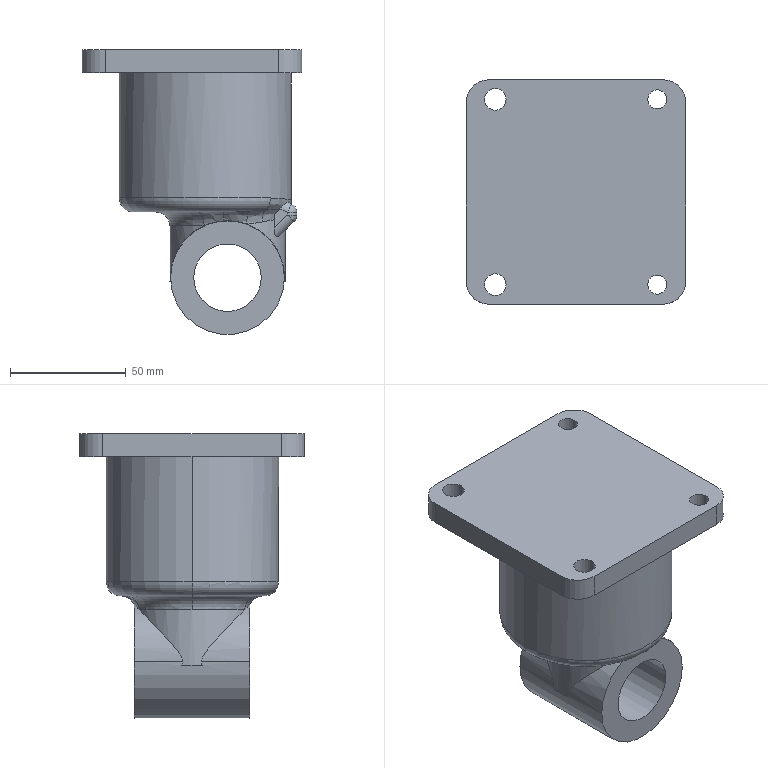Part | SolidWorks | features Fillet 5, ICE 5, Extrusion 1 | 1 solid | 65 faces | box 95 x 97 x 123 mm | volume 427032 mm3 | cylinder 30 | plane 18 | spline 9 | torus 4 | sphere 4 | commonest cylinder face diameters 8 x8 8.196 x4 9.372 x4 20 x4 49.179 x3 49.876 x3